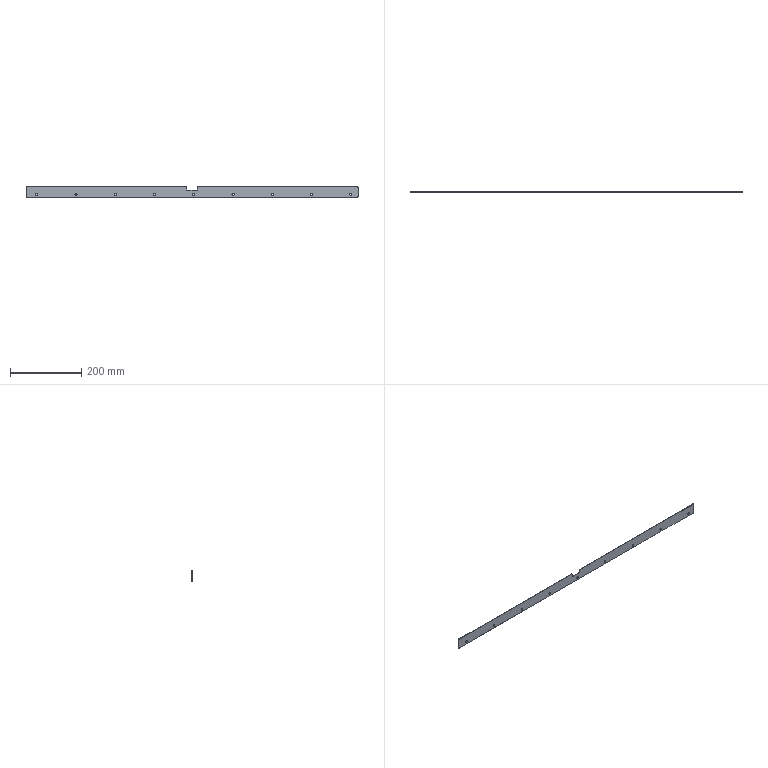Part | NX | features solid 2 | 1 solid | 34 faces | box 930 x 1.5 x 30 mm | volume 41011 mm3 | cylinder 24 | plane 10 | commonest cylinder face diameters 6 x18 4 x6
STEP:
#1=CARTESIAN_POINT('',(629.,-1449.,118.844));
#2=VERTEX_POINT('',#1);
#3=CARTESIAN_POINT('',(631.,-1449.,116.844));
#4=VERTEX_POINT('',#3);
#5=CARTESIAN_POINT('',(629.,-1449.,116.844));
#6=DIRECTION('',(0.,1.,0.));
#7=DIRECTION('',(-1.,0.,0.));
#8=AXIS2_PLACEMENT_3D('',#5,#6,#7);
#9=CIRCLE('',#8,2.);
#10=EDGE_CURVE('',#2,#4,#9,.T.);
#11=ORIENTED_EDGE('',*,*,#10,.F.);
#12=CARTESIAN_POINT('',(629.,-1450.5,118.844));
#13=VERTEX_POINT('',#12);
#14=CARTESIAN_POINT('',(629.,-1449.,118.844));
#15=DIRECTION('',(0.,1.,0.));
#16=VECTOR('',#15,1000.);
#17=LINE('',#14,#16);
#18=EDGE_CURVE('',#13,#2,#17,.T.);
#19=ORIENTED_EDGE('',*,*,#18,.F.);
#20=CARTESIAN_POINT('',(631.,-1450.5,116.844));
#21=VERTEX_POINT('',#20);
#22=CARTESIAN_POINT('',(629.,-1450.5,116.844));
#23=DIRECTION('',(0.,-1.,0.));
#24=DIRECTION('',(-1.,0.,0.));
#25=AXIS2_PLACEMENT_3D('',#22,#23,#24);
#26=CIRCLE('',#25,2.);
#27=EDGE_CURVE('',#21,#13,#26,.T.);
#28=ORIENTED_EDGE('',*,*,#27,.F.);
#29=CARTESIAN_POINT('',(631.,-1449.,116.844));
#30=DIRECTION('',(0.,-1.,0.));
#31=VECTOR('',#30,1000.);
#32=LINE('',#29,#31);
#33=EDGE_CURVE('',#4,#21,#32,.T.);
#34=ORIENTED_EDGE('',*,*,#33,.F.);
#35=EDGE_LOOP('',(#11,#19,#28,#34));
#36=FACE_BOUND('',#35,.T.);
#37=CARTESIAN_POINT('',(629.,-1449.,116.844));
#38=DIRECTION('',(0.,-1.,0.));
#39=DIRECTION('',(0.,0.,-1.));
#40=AXIS2_PLACEMENT_3D('',#37,#38,#39);
#41=CYLINDRICAL_SURFACE('',#40,2.);
#42=ADVANCED_FACE('',(#36),#41,.T.);
#43=CARTESIAN_POINT('',(631.,-1449.,90.844));
#44=VERTEX_POINT('',#43);
#45=CARTESIAN_POINT('',(629.,-1449.,88.844));
#46=VERTEX_POINT('',#45);
#47=CARTESIAN_POINT('',(629.,-1449.,90.844));
#48=DIRECTION('',(0.,1.,0.));
#49=DIRECTION('',(-1.,0.,0.));
#50=AXIS2_PLACEMENT_3D('',#47,#48,#49);
#51=CIRCLE('',#50,2.);
#52=EDGE_CURVE('',#44,#46,#51,.T.);
#53=ORIENTED_EDGE('',*,*,#52,.F.);
#54=CARTESIAN_POINT('',(631.,-1450.5,90.844));
#55=VERTEX_POINT('',#54);
#56=CARTESIAN_POINT('',(631.,-1449.,90.844));
#57=DIRECTION('',(0.,1.,0.));
#58=VECTOR('',#57,1000.);
#59=LINE('',#56,#58);
#60=EDGE_CURVE('',#55,#44,#59,.T.);
#61=ORIENTED_EDGE('',*,*,#60,.F.);
#62=CARTESIAN_POINT('',(629.,-1450.5,88.844));
#63=VERTEX_POINT('',#62);
#64=CARTESIAN_POINT('',(629.,-1450.5,90.844));
#65=DIRECTION('',(0.,-1.,0.));
#66=DIRECTION('',(-1.,0.,0.));
#67=AXIS2_PLACEMENT_3D('',#64,#65,#66);
#68=CIRCLE('',#67,2.);
#69=EDGE_CURVE('',#63,#55,#68,.T.);
#70=ORIENTED_EDGE('',*,*,#69,.F.);
#71=CARTESIAN_POINT('',(629.,-1449.,88.844));
#72=DIRECTION('',(0.,-1.,0.));
#73=VECTOR('',#72,1000.);
#74=LINE('',#71,#73);
#75=EDGE_CURVE('',#46,#63,#74,.T.);
#76=ORIENTED_EDGE('',*,*,#75,.F.);
#77=EDGE_LOOP('',(#53,#61,#70,#76));
#78=FACE_BOUND('',#77,.T.);
#79=CARTESIAN_POINT('',(629.,-1449.,90.844));
#80=DIRECTION('',(0.,-1.,0.));
#81=DIRECTION('',(0.,0.,-1.));
#82=AXIS2_PLACEMENT_3D('',#79,#80,#81);
#83=CYLINDRICAL_SURFACE('',#82,2.);
#84=ADVANCED_FACE('',(#78),#83,.T.);
#85=CARTESIAN_POINT('',(149.,-1449.,118.844));
#86=VERTEX_POINT('',#85);
#87=CARTESIAN_POINT('',(151.,-1449.,116.844));
#88=VERTEX_POINT('',#87);
#89=CARTESIAN_POINT('',(149.,-1449.,116.844));
#90=DIRECTION('',(0.,1.,0.));
#91=DIRECTION('',(-1.,0.,0.));
#92=AXIS2_PLACEMENT_3D('',#89,#90,#91);
#93=CIRCLE('',#92,2.);
#94=EDGE_CURVE('',#86,#88,#93,.T.);
#95=ORIENTED_EDGE('',*,*,#94,.F.);
#96=CARTESIAN_POINT('',(149.,-1450.5,118.844));
#97=VERTEX_POINT('',#96);
#98=CARTESIAN_POINT('',(149.,-1449.,118.844));
#99=DIRECTION('',(0.,1.,0.));
#100=VECTOR('',#99,1000.);
#101=LINE('',#98,#100);
#102=EDGE_CURVE('',#97,#86,#101,.T.);
#103=ORIENTED_EDGE('',*,*,#102,.F.);
#104=CARTESIAN_POINT('',(151.,-1450.5,116.844));
#105=VERTEX_POINT('',#104);
#106=CARTESIAN_POINT('',(149.,-1450.5,116.844));
#107=DIRECTION('',(0.,-1.,0.));
#108=DIRECTION('',(-1.,0.,0.));
#109=AXIS2_PLACEMENT_3D('',#106,#107,#108);
#110=CIRCLE('',#109,2.);
#111=EDGE_CURVE('',#105,#97,#110,.T.);
#112=ORIENTED_EDGE('',*,*,#111,.F.);
#113=CARTESIAN_POINT('',(151.,-1450.5,116.844));
#114=DIRECTION('',(0.,-1.,0.));
#115=VECTOR('',#114,1000.);
#116=LINE('',#113,#115);
#117=EDGE_CURVE('',#88,#105,#116,.T.);
#118=ORIENTED_EDGE('',*,*,#117,.F.);
#119=EDGE_LOOP('',(#95,#103,#112,#118));
#120=FACE_BOUND('',#119,.T.);
#121=CARTESIAN_POINT('',(149.,-1450.5,116.844));
#122=DIRECTION('',(0.,-1.,0.));
#123=DIRECTION('',(1.,0.,0.));
#124=AXIS2_PLACEMENT_3D('',#121,#122,#123);
#125=CYLINDRICAL_SURFACE('',#124,2.);
#126=ADVANCED_FACE('',(#120),#125,.T.);
#127=CARTESIAN_POINT('',(181.,-1449.,116.844));
#128=VERTEX_POINT('',#127);
#129=CARTESIAN_POINT('',(183.,-1449.,118.844));
#130=VERTEX_POINT('',#129);
#131=CARTESIAN_POINT('',(183.,-1449.,116.844));
#132=DIRECTION('',(0.,1.,0.));
#133=DIRECTION('',(-1.,0.,0.));
#134=AXIS2_PLACEMENT_3D('',#131,#132,#133);
#135=CIRCLE('',#134,2.);
#136=EDGE_CURVE('',#128,#130,#135,.T.);
#137=ORIENTED_EDGE('',*,*,#136,.F.);
#138=CARTESIAN_POINT('',(181.,-1450.5,116.844));
#139=VERTEX_POINT('',#138);
#140=CARTESIAN_POINT('',(181.,-1450.5,116.844));
#141=DIRECTION('',(0.,1.,0.));
#142=VECTOR('',#141,1000.);
#143=LINE('',#140,#142);
#144=EDGE_CURVE('',#139,#128,#143,.T.);
#145=ORIENTED_EDGE('',*,*,#144,.F.);
#146=CARTESIAN_POINT('',(183.,-1450.5,118.844));
#147=VERTEX_POINT('',#146);
#148=CARTESIAN_POINT('',(183.,-1450.5,116.844));
#149=DIRECTION('',(0.,-1.,0.));
#150=DIRECTION('',(-1.,0.,0.));
#151=AXIS2_PLACEMENT_3D('',#148,#149,#150);
#152=CIRCLE('',#151,2.);
#153=EDGE_CURVE('',#147,#139,#152,.T.);
#154=ORIENTED_EDGE('',*,*,#153,.F.);
#155=CARTESIAN_POINT('',(183.,-1449.,118.844));
#156=DIRECTION('',(0.,-1.,0.));
#157=VECTOR('',#156,1000.);
#158=LINE('',#155,#157);
#159=EDGE_CURVE('',#130,#147,#158,.T.);
#160=ORIENTED_EDGE('',*,*,#159,.F.);
#161=EDGE_LOOP('',(#137,#145,#154,#160));
#162=FACE_BOUND('',#161,.T.);
#163=CARTESIAN_POINT('',(183.,-1449.,116.844));
#164=DIRECTION('',(0.,-1.,0.));
#165=DIRECTION('',(1.,0.,0.));
#166=AXIS2_PLACEMENT_3D('',#163,#164,#165);
#167=CYLINDRICAL_SURFACE('',#166,2.);
#168=ADVANCED_FACE('',(#162),#167,.T.);
#169=CARTESIAN_POINT('',(-299.,-1449.,116.844));
#170=VERTEX_POINT('',#169);
#171=CARTESIAN_POINT('',(-297.,-1449.,118.844));
#172=VERTEX_POINT('',#171);
#173=CARTESIAN_POINT('',(-297.,-1449.,116.844));
#174=DIRECTION('',(0.,1.,0.));
#175=DIRECTION('',(-1.,0.,0.));
#176=AXIS2_PLACEMENT_3D('',#173,#174,#175);
#177=CIRCLE('',#176,2.);
#178=EDGE_CURVE('',#170,#172,#177,.T.);
#179=ORIENTED_EDGE('',*,*,#178,.F.);
#180=CARTESIAN_POINT('',(-299.,-1450.5,116.844));
#181=VERTEX_POINT('',#180);
#182=CARTESIAN_POINT('',(-299.,-1449.,116.844));
#183=DIRECTION('',(0.,1.,0.));
#184=VECTOR('',#183,1000.);
#185=LINE('',#182,#184);
#186=EDGE_CURVE('',#181,#170,#185,.T.);
#187=ORIENTED_EDGE('',*,*,#186,.F.);
#188=CARTESIAN_POINT('',(-297.,-1450.5,118.844));
#189=VERTEX_POINT('',#188);
#190=CARTESIAN_POINT('',(-297.,-1450.5,116.844));
#191=DIRECTION('',(0.,-1.,0.));
#192=DIRECTION('',(-1.,0.,0.));
#193=AXIS2_PLACEMENT_3D('',#190,#191,#192);
#194=CIRCLE('',#193,2.);
#195=EDGE_CURVE('',#189,#181,#194,.T.);
#196=ORIENTED_EDGE('',*,*,#195,.F.);
#197=CARTESIAN_POINT('',(-297.,-1449.,118.844));
#198=DIRECTION('',(0.,-1.,0.));
#199=VECTOR('',#198,1000.);
#200=LINE('',#197,#199);
#201=EDGE_CURVE('',#172,#189,#200,.T.);
#202=ORIENTED_EDGE('',*,*,#201,.F.);
#203=EDGE_LOOP('',(#179,#187,#196,#202));
#204=FACE_BOUND('',#203,.T.);
#205=CARTESIAN_POINT('',(-297.,-1449.,116.844));
#206=DIRECTION('',(0.,-1.,0.));
#207=DIRECTION('',(0.,0.,-1.));
#208=AXIS2_PLACEMENT_3D('',#205,#206,#207);
#209=CYLINDRICAL_SURFACE('',#208,2.);
#210=ADVANCED_FACE('',(#204),#209,.T.);
#211=CARTESIAN_POINT('',(-297.,-1449.,88.844));
#212=VERTEX_POINT('',#211);
#213=CARTESIAN_POINT('',(-299.,-1449.,90.844));
#214=VERTEX_POINT('',#213);
#215=CARTESIAN_POINT('',(-297.,-1449.,90.844));
#216=DIRECTION('',(0.,1.,0.));
#217=DIRECTION('',(-1.,0.,0.));
#218=AXIS2_PLACEMENT_3D('',#215,#216,#217);
#219=CIRCLE('',#218,2.);
#220=EDGE_CURVE('',#212,#214,#219,.T.);
#221=ORIENTED_EDGE('',*,*,#220,.F.);
#222=CARTESIAN_POINT('',(-297.,-1450.5,88.844));
#223=VERTEX_POINT('',#222);
#224=CARTESIAN_POINT('',(-297.,-1449.,88.844));
#225=DIRECTION('',(0.,1.,0.));
#226=VECTOR('',#225,1000.);
#227=LINE('',#224,#226);
#228=EDGE_CURVE('',#223,#212,#227,.T.);
#229=ORIENTED_EDGE('',*,*,#228,.F.);
#230=CARTESIAN_POINT('',(-299.,-1450.5,90.844));
#231=VERTEX_POINT('',#230);
#232=CARTESIAN_POINT('',(-297.,-1450.5,90.844));
#233=DIRECTION('',(0.,-1.,0.));
#234=DIRECTION('',(-1.,0.,0.));
#235=AXIS2_PLACEMENT_3D('',#232,#233,#234);
#236=CIRCLE('',#235,2.);
#237=EDGE_CURVE('',#231,#223,#236,.T.);
#238=ORIENTED_EDGE('',*,*,#237,.F.);
#239=CARTESIAN_POINT('',(-299.,-1449.,90.844));
#240=DIRECTION('',(0.,-1.,0.));
#241=VECTOR('',#240,1000.);
#242=LINE('',#239,#241);
#243=EDGE_CURVE('',#214,#231,#242,.T.);
#244=ORIENTED_EDGE('',*,*,#243,.F.);
#245=EDGE_LOOP('',(#221,#229,#238,#244));
#246=FACE_BOUND('',#245,.T.);
#247=CARTESIAN_POINT('',(-297.,-1449.,90.844));
#248=DIRECTION('',(0.,-1.,0.));
#249=DIRECTION('',(0.,0.,-1.));
#250=AXIS2_PLACEMENT_3D('',#247,#248,#249);
#251=CYLINDRICAL_SURFACE('',#250,2.);
#252=ADVANCED_FACE('',(#246),#251,.T.);
#253=CARTESIAN_POINT('',(-266.,-1450.5,97.344));
#254=VERTEX_POINT('',#253);
#255=CARTESIAN_POINT('',(-266.,-1449.,97.344));
#256=VERTEX_POINT('',#255);
#257=CARTESIAN_POINT('',(-266.,-2379.485,97.344));
#258=DIRECTION('',(0.,1.,0.));
#259=VECTOR('',#258,1000.);
#260=LINE('',#257,#259);
#261=EDGE_CURVE('',#254,#256,#260,.T.);
#262=ORIENTED_EDGE('',*,*,#261,.F.);
#263=CARTESIAN_POINT('',(-272.,-1450.5,97.344));
#264=VERTEX_POINT('',#263);
#265=CARTESIAN_POINT('',(-269.,-1450.5,97.344));
#266=DIRECTION('',(0.,1.,0.));
#267=DIRECTION('',(-1.,0.,0.));
#268=AXIS2_PLACEMENT_3D('',#265,#266,#267);
#269=CIRCLE('',#268,3.);
#270=EDGE_CURVE('',#264,#254,#269,.T.);
#271=ORIENTED_EDGE('',*,*,#270,.F.);
#272=CARTESIAN_POINT('',(-272.,-1449.,97.344));
#273=VERTEX_POINT('',#272);
#274=CARTESIAN_POINT('',(-272.,-2379.485,97.344));
#275=DIRECTION('',(0.,1.,0.));
#276=VECTOR('',#275,1000.);
#277=LINE('',#274,#276);
#278=EDGE_CURVE('',#273,#264,#277,.F.);
#279=ORIENTED_EDGE('',*,*,#278,.F.);
#280=CARTESIAN_POINT('',(-269.,-1449.,97.344));
#281=DIRECTION('',(0.,1.,0.));
#282=DIRECTION('',(-1.,0.,0.));
#283=AXIS2_PLACEMENT_3D('',#280,#281,#282);
#284=CIRCLE('',#283,3.);
#285=EDGE_CURVE('',#273,#256,#284,.T.);
#286=ORIENTED_EDGE('',*,*,#285,.T.);
#287=EDGE_LOOP('',(#262,#271,#279,#286));
#288=FACE_BOUND('',#287,.T.);
#289=CARTESIAN_POINT('',(-269.,-2379.485,97.344));
#290=DIRECTION('',(0.,1.,0.));
#291=DIRECTION('',(-1.,0.,0.));
#292=AXIS2_PLACEMENT_3D('',#289,#290,#291);
#293=CYLINDRICAL_SURFACE('',#292,3.);
#294=ADVANCED_FACE('',(#288),#293,.F.);
#295=CARTESIAN_POINT('',(-156.,-1450.5,97.344));
#296=VERTEX_POINT('',#295);
#297=CARTESIAN_POINT('',(-156.,-1449.,97.344));
#298=VERTEX_POINT('',#297);
#299=CARTESIAN_POINT('',(-156.,-2379.485,97.344));
#300=DIRECTION('',(0.,1.,0.));
#301=VECTOR('',#300,1000.);
#302=LINE('',#299,#301);
#303=EDGE_CURVE('',#296,#298,#302,.T.);
#304=ORIENTED_EDGE('',*,*,#303,.F.);
#305=CARTESIAN_POINT('',(-162.,-1450.5,97.344));
#306=VERTEX_POINT('',#305);
#307=CARTESIAN_POINT('',(-159.,-1450.5,97.344));
#308=DIRECTION('',(0.,1.,0.));
#309=DIRECTION('',(-1.,0.,0.));
#310=AXIS2_PLACEMENT_3D('',#307,#308,#309);
#311=CIRCLE('',#310,3.);
#312=EDGE_CURVE('',#306,#296,#311,.T.);
#313=ORIENTED_EDGE('',*,*,#312,.F.);
#314=CARTESIAN_POINT('',(-162.,-1449.,97.344));
#315=VERTEX_POINT('',#314);
#316=CARTESIAN_POINT('',(-162.,-2379.485,97.344));
#317=DIRECTION('',(0.,1.,0.));
#318=VECTOR('',#317,1000.);
#319=LINE('',#316,#318);
#320=EDGE_CURVE('',#315,#306,#319,.F.);
#321=ORIENTED_EDGE('',*,*,#320,.F.);
#322=CARTESIAN_POINT('',(-159.,-1449.,97.344));
#323=DIRECTION('',(0.,1.,0.));
#324=DIRECTION('',(-1.,0.,0.));
#325=AXIS2_PLACEMENT_3D('',#322,#323,#324);
#326=CIRCLE('',#325,3.);
#327=EDGE_CURVE('',#315,#298,#326,.T.);
#328=ORIENTED_EDGE('',*,*,#327,.T.);
#329=EDGE_LOOP('',(#304,#313,#321,#328));
#330=FACE_BOUND('',#329,.T.);
#331=CARTESIAN_POINT('',(-159.,-2379.485,97.344));
#332=DIRECTION('',(0.,1.,0.));
#333=DIRECTION('',(-1.,0.,0.));
#334=AXIS2_PLACEMENT_3D('',#331,#332,#333);
#335=CYLINDRICAL_SURFACE('',#334,3.);
#336=ADVANCED_FACE('',(#330),#335,.F.);
#337=CARTESIAN_POINT('',(-46.,-1449.,97.344));
#338=VERTEX_POINT('',#337);
#339=CARTESIAN_POINT('',(-46.,-1450.5,97.344));
#340=VERTEX_POINT('',#339);
#341=CARTESIAN_POINT('',(-46.,-2379.485,97.344));
#342=DIRECTION('',(0.,1.,0.));
#343=VECTOR('',#342,1000.);
#344=LINE('',#341,#343);
#345=EDGE_CURVE('',#338,#340,#344,.F.);
#346=ORIENTED_EDGE('',*,*,#345,.T.);
#347=CARTESIAN_POINT('',(-52.,-1450.5,97.344));
#348=VERTEX_POINT('',#347);
#349=CARTESIAN_POINT('',(-49.,-1450.5,97.344));
#350=DIRECTION('',(0.,1.,0.));
#351=DIRECTION('',(-1.,0.,0.));
#352=AXIS2_PLACEMENT_3D('',#349,#350,#351);
#353=CIRCLE('',#352,3.);
#354=EDGE_CURVE('',#348,#340,#353,.T.);
#355=ORIENTED_EDGE('',*,*,#354,.F.);
#356=CARTESIAN_POINT('',(-52.,-1449.,97.344));
#357=VERTEX_POINT('',#356);
#358=CARTESIAN_POINT('',(-52.,-2379.485,97.344));
#359=DIRECTION('',(0.,1.,0.));
#360=VECTOR('',#359,1000.);
#361=LINE('',#358,#360);
#362=EDGE_CURVE('',#348,#357,#361,.T.);
#363=ORIENTED_EDGE('',*,*,#362,.T.);
#364=CARTESIAN_POINT('',(-49.,-1449.,97.344));
#365=DIRECTION('',(0.,1.,0.));
#366=DIRECTION('',(-1.,0.,0.));
#367=AXIS2_PLACEMENT_3D('',#364,#365,#366);
#368=CIRCLE('',#367,3.);
#369=EDGE_CURVE('',#357,#338,#368,.T.);
#370=ORIENTED_EDGE('',*,*,#369,.T.);
#371=EDGE_LOOP('',(#346,#355,#363,#370));
#372=FACE_BOUND('',#371,.T.);
#373=CARTESIAN_POINT('',(-49.,-2379.485,97.344));
#374=DIRECTION('',(0.,1.,0.));
#375=DIRECTION('',(-1.,0.,0.));
#376=AXIS2_PLACEMENT_3D('',#373,#374,#375);
#377=CYLINDRICAL_SURFACE('',#376,3.);
#378=ADVANCED_FACE('',(#372),#377,.F.);
#379=CARTESIAN_POINT('',(64.,-1450.5,97.344));
#380=VERTEX_POINT('',#379);
#381=CARTESIAN_POINT('',(64.,-1449.,97.344));
#382=VERTEX_POINT('',#381);
#383=CARTESIAN_POINT('',(64.,-2379.485,97.344));
#384=DIRECTION('',(0.,1.,0.));
#385=VECTOR('',#384,1000.);
#386=LINE('',#383,#385);
#387=EDGE_CURVE('',#380,#382,#386,.T.);
#388=ORIENTED_EDGE('',*,*,#387,.F.);
#389=CARTESIAN_POINT('',(58.,-1450.5,97.344));
#390=VERTEX_POINT('',#389);
#391=CARTESIAN_POINT('',(61.,-1450.5,97.344));
#392=DIRECTION('',(0.,1.,0.));
#393=DIRECTION('',(-1.,0.,0.));
#394=AXIS2_PLACEMENT_3D('',#391,#392,#393);
#395=CIRCLE('',#394,3.);
#396=EDGE_CURVE('',#390,#380,#395,.T.);
#397=ORIENTED_EDGE('',*,*,#396,.F.);
#398=CARTESIAN_POINT('',(58.,-1449.,97.344));
#399=VERTEX_POINT('',#398);
#400=CARTESIAN_POINT('',(58.,-2379.485,97.344));
#401=DIRECTION('',(0.,1.,0.));
#402=VECTOR('',#401,1000.);
#403=LINE('',#400,#402);
#404=EDGE_CURVE('',#399,#390,#403,.F.);
#405=ORIENTED_EDGE('',*,*,#404,.F.);
#406=CARTESIAN_POINT('',(61.,-1449.,97.344));
#407=DIRECTION('',(0.,1.,0.));
#408=DIRECTION('',(-1.,0.,0.));
#409=AXIS2_PLACEMENT_3D('',#406,#407,#408);
#410=CIRCLE('',#409,3.);
#411=EDGE_CURVE('',#399,#382,#410,.T.);
#412=ORIENTED_EDGE('',*,*,#411,.T.);
#413=EDGE_LOOP('',(#388,#397,#405,#412));
#414=FACE_BOUND('',#413,.T.);
#415=CARTESIAN_POINT('',(61.,-2379.485,97.344));
#416=DIRECTION('',(0.,1.,0.));
#417=DIRECTION('',(-1.,0.,0.));
#418=AXIS2_PLACEMENT_3D('',#415,#416,#417);
#419=CYLINDRICAL_SURFACE('',#418,3.);
#420=ADVANCED_FACE('',(#414),#419,.F.);
#421=CARTESIAN_POINT('',(174.,-1450.5,97.344));
#422=VERTEX_POINT('',#421);
#423=CARTESIAN_POINT('',(174.,-1449.,97.344));
#424=VERTEX_POINT('',#423);
#425=CARTESIAN_POINT('',(174.,-2379.485,97.344));
#426=DIRECTION('',(0.,1.,0.));
#427=VECTOR('',#426,1000.);
#428=LINE('',#425,#427);
#429=EDGE_CURVE('',#422,#424,#428,.T.);
#430=ORIENTED_EDGE('',*,*,#429,.F.);
#431=CARTESIAN_POINT('',(168.,-1450.5,97.344));
#432=VERTEX_POINT('',#431);
#433=CARTESIAN_POINT('',(171.,-1450.5,97.344));
#434=DIRECTION('',(0.,1.,0.));
#435=DIRECTION('',(-1.,0.,0.));
#436=AXIS2_PLACEMENT_3D('',#433,#434,#435);
#437=CIRCLE('',#436,3.);
#438=EDGE_CURVE('',#432,#422,#437,.T.);
#439=ORIENTED_EDGE('',*,*,#438,.F.);
#440=CARTESIAN_POINT('',(168.,-1449.,97.344));
#441=VERTEX_POINT('',#440);
#442=CARTESIAN_POINT('',(168.,-2379.485,97.344));
#443=DIRECTION('',(0.,1.,0.));
#444=VECTOR('',#443,1000.);
#445=LINE('',#442,#444);
#446=EDGE_CURVE('',#441,#432,#445,.F.);
#447=ORIENTED_EDGE('',*,*,#446,.F.);
#448=CARTESIAN_POINT('',(171.,-1449.,97.344));
#449=DIRECTION('',(0.,1.,0.));
#450=DIRECTION('',(-1.,0.,0.));
#451=AXIS2_PLACEMENT_3D('',#448,#449,#450);
#452=CIRCLE('',#451,3.);
#453=EDGE_CURVE('',#441,#424,#452,.T.);
#454=ORIENTED_EDGE('',*,*,#453,.T.);
#455=EDGE_LOOP('',(#430,#439,#447,#454));
#456=FACE_BOUND('',#455,.T.);
#457=CARTESIAN_POINT('',(171.,-2379.485,97.344));
#458=DIRECTION('',(0.,1.,0.));
#459=DIRECTION('',(-1.,0.,0.));
#460=AXIS2_PLACEMENT_3D('',#457,#458,#459);
#461=CYLINDRICAL_SURFACE('',#460,3.);
#462=ADVANCED_FACE('',(#456),#461,.F.);
#463=CARTESIAN_POINT('',(284.,-1449.,97.344));
#464=VERTEX_POINT('',#463);
#465=CARTESIAN_POINT('',(284.,-1450.5,97.344));
#466=VERTEX_POINT('',#465);
#467=CARTESIAN_POINT('',(284.,-2379.485,97.344));
#468=DIRECTION('',(0.,1.,0.));
#469=VECTOR('',#468,1000.);
#470=LINE('',#467,#469);
#471=EDGE_CURVE('',#464,#466,#470,.F.);
#472=ORIENTED_EDGE('',*,*,#471,.T.);
#473=CARTESIAN_POINT('',(278.,-1450.5,97.344));
#474=VERTEX_POINT('',#473);
#475=CARTESIAN_POINT('',(281.,-1450.5,97.344));
#476=DIRECTION('',(0.,1.,0.));
#477=DIRECTION('',(-1.,0.,0.));
#478=AXIS2_PLACEMENT_3D('',#475,#476,#477);
#479=CIRCLE('',#478,3.);
#480=EDGE_CURVE('',#474,#466,#479,.T.);
#481=ORIENTED_EDGE('',*,*,#480,.F.);
#482=CARTESIAN_POINT('',(278.,-1449.,97.344));
#483=VERTEX_POINT('',#482);
#484=CARTESIAN_POINT('',(278.,-2379.485,97.344));
#485=DIRECTION('',(0.,1.,0.));
#486=VECTOR('',#485,1000.);
#487=LINE('',#484,#486);
#488=EDGE_CURVE('',#474,#483,#487,.T.);
#489=ORIENTED_EDGE('',*,*,#488,.T.);
#490=CARTESIAN_POINT('',(281.,-1449.,97.344));
#491=DIRECTION('',(0.,1.,0.));
#492=DIRECTION('',(-1.,0.,0.));
#493=AXIS2_PLACEMENT_3D('',#490,#491,#492);
#494=CIRCLE('',#493,3.);
#495=EDGE_CURVE('',#483,#464,#494,.T.);
#496=ORIENTED_EDGE('',*,*,#495,.T.);
#497=EDGE_LOOP('',(#472,#481,#489,#496));
#498=FACE_BOUND('',#497,.T.);
#499=CARTESIAN_POINT('',(281.,-2379.485,97.344));
#500=DIRECTION('',(0.,1.,0.));
#501=DIRECTION('',(-1.,0.,0.));
#502=AXIS2_PLACEMENT_3D('',#499,#500,#501);
#503=CYLINDRICAL_SURFACE('',#502,3.);
#504=ADVANCED_FACE('',(#498),#503,.F.);
#505=CARTESIAN_POINT('',(394.,-1450.5,97.344));
#506=VERTEX_POINT('',#505);
#507=CARTESIAN_POINT('',(394.,-1449.,97.344));
#508=VERTEX_POINT('',#507);
#509=CARTESIAN_POINT('',(394.,-2379.485,97.344));
#510=DIRECTION('',(0.,1.,0.));
#511=VECTOR('',#510,1000.);
#512=LINE('',#509,#511);
#513=EDGE_CURVE('',#506,#508,#512,.T.);
#514=ORIENTED_EDGE('',*,*,#513,.F.);
#515=CARTESIAN_POINT('',(388.,-1450.5,97.344));
#516=VERTEX_POINT('',#515);
#517=CARTESIAN_POINT('',(391.,-1450.5,97.344));
#518=DIRECTION('',(0.,1.,0.));
#519=DIRECTION('',(-1.,0.,0.));
#520=AXIS2_PLACEMENT_3D('',#517,#518,#519);
#521=CIRCLE('',#520,3.);
#522=EDGE_CURVE('',#516,#506,#521,.T.);
#523=ORIENTED_EDGE('',*,*,#522,.F.);
#524=CARTESIAN_POINT('',(388.,-1449.,97.344));
#525=VERTEX_POINT('',#524);
#526=CARTESIAN_POINT('',(388.,-2379.485,97.344));
#527=DIRECTION('',(0.,1.,0.));
#528=VECTOR('',#527,1000.);
#529=LINE('',#526,#528);
#530=EDGE_CURVE('',#525,#516,#529,.F.);
#531=ORIENTED_EDGE('',*,*,#530,.F.);
#532=CARTESIAN_POINT('',(391.,-1449.,97.344));
#533=DIRECTION('',(0.,1.,0.));
#534=DIRECTION('',(-1.,0.,0.));
#535=AXIS2_PLACEMENT_3D('',#532,#533,#534);
#536=CIRCLE('',#535,3.);
#537=EDGE_CURVE('',#525,#508,#536,.T.);
#538=ORIENTED_EDGE('',*,*,#537,.T.);
#539=EDGE_LOOP('',(#514,#523,#531,#538));
#540=FACE_BOUND('',#539,.T.);
#541=CARTESIAN_POINT('',(391.,-2379.485,97.344));
#542=DIRECTION('',(0.,1.,0.));
#543=DIRECTION('',(-1.,0.,0.));
#544=AXIS2_PLACEMENT_3D('',#541,#542,#543);
#545=CYLINDRICAL_SURFACE('',#544,3.);
#546=ADVANCED_FACE('',(#540),#545,.F.);
#547=CARTESIAN_POINT('',(504.,-1449.,97.344));
#548=VERTEX_POINT('',#547);
#549=CARTESIAN_POINT('',(504.,-1450.5,97.344));
#550=VERTEX_POINT('',#549);
#551=CARTESIAN_POINT('',(504.,-2379.485,97.344));
#552=DIRECTION('',(0.,1.,0.));
#553=VECTOR('',#552,1000.);
#554=LINE('',#551,#553);
#555=EDGE_CURVE('',#548,#550,#554,.F.);
#556=ORIENTED_EDGE('',*,*,#555,.T.);
#557=CARTESIAN_POINT('',(498.,-1450.5,97.344));
#558=VERTEX_POINT('',#557);
#559=CARTESIAN_POINT('',(501.,-1450.5,97.344));
#560=DIRECTION('',(0.,1.,0.));
#561=DIRECTION('',(-1.,0.,0.));
#562=AXIS2_PLACEMENT_3D('',#559,#560,#561);
#563=CIRCLE('',#562,3.);
#564=EDGE_CURVE('',#558,#550,#563,.T.);
#565=ORIENTED_EDGE('',*,*,#564,.F.);
#566=CARTESIAN_POINT('',(498.,-1449.,97.344));
#567=VERTEX_POINT('',#566);
#568=CARTESIAN_POINT('',(498.,-2379.485,97.344));
#569=DIRECTION('',(0.,1.,0.));
#570=VECTOR('',#569,1000.);
#571=LINE('',#568,#570);
#572=EDGE_CURVE('',#558,#567,#571,.T.);
#573=ORIENTED_EDGE('',*,*,#572,.T.);
#574=CARTESIAN_POINT('',(501.,-1449.,97.344));
#575=DIRECTION('',(0.,1.,0.));
#576=DIRECTION('',(-1.,0.,0.));
#577=AXIS2_PLACEMENT_3D('',#574,#575,#576);
#578=CIRCLE('',#577,3.);
#579=EDGE_CURVE('',#567,#548,#578,.T.);
#580=ORIENTED_EDGE('',*,*,#579,.T.);
#581=EDGE_LOOP('',(#556,#565,#573,#580));
#582=FACE_BOUND('',#581,.T.);
#583=CARTESIAN_POINT('',(501.,-2379.485,97.344));
#584=DIRECTION('',(0.,1.,0.));
#585=DIRECTION('',(-1.,0.,0.));
#586=AXIS2_PLACEMENT_3D('',#583,#584,#585);
#587=CYLINDRICAL_SURFACE('',#586,3.);
#588=ADVANCED_FACE('',(#582),#587,.F.);
#589=CARTESIAN_POINT('',(614.,-1450.5,97.344));
#590=VERTEX_POINT('',#589);
#591=CARTESIAN_POINT('',(614.,-1449.,97.344));
#592=VERTEX_POINT('',#591);
#593=CARTESIAN_POINT('',(614.,-2379.485,97.344));
#594=DIRECTION('',(0.,1.,0.));
#595=VECTOR('',#594,1000.);
#596=LINE('',#593,#595);
#597=EDGE_CURVE('',#590,#592,#596,.T.);
#598=ORIENTED_EDGE('',*,*,#597,.F.);
#599=CARTESIAN_POINT('',(608.,-1450.5,97.344));
#600=VERTEX_POINT('',#599);
#601=CARTESIAN_POINT('',(611.,-1450.5,97.344));
#602=DIRECTION('',(0.,1.,0.));
#603=DIRECTION('',(-1.,0.,0.));
#604=AXIS2_PLACEMENT_3D('',#601,#602,#603);
#605=CIRCLE('',#604,3.);
#606=EDGE_CURVE('',#600,#590,#605,.T.);
#607=ORIENTED_EDGE('',*,*,#606,.F.);
#608=CARTESIAN_POINT('',(608.,-1449.,97.344));
#609=VERTEX_POINT('',#608);
#610=CARTESIAN_POINT('',(608.,-2379.485,97.344));
#611=DIRECTION('',(0.,1.,0.));
#612=VECTOR('',#611,1000.);
#613=LINE('',#610,#612);
#614=EDGE_CURVE('',#609,#600,#613,.F.);
#615=ORIENTED_EDGE('',*,*,#614,.F.);
#616=CARTESIAN_POINT('',(611.,-1449.,97.344));
#617=DIRECTION('',(0.,1.,0.));
#618=DIRECTION('',(-1.,0.,0.));
#619=AXIS2_PLACEMENT_3D('',#616,#617,#618);
#620=CIRCLE('',#619,3.);
#621=EDGE_CURVE('',#609,#592,#620,.T.);
#622=ORIENTED_EDGE('',*,*,#621,.T.);
#623=EDGE_LOOP('',(#598,#607,#615,#622));
#624=FACE_BOUND('',#623,.T.);
#625=CARTESIAN_POINT('',(611.,-2379.485,97.344));
#626=DIRECTION('',(0.,1.,0.));
#627=DIRECTION('',(-1.,0.,0.));
#628=AXIS2_PLACEMENT_3D('',#625,#626,#627);
#629=CYLINDRICAL_SURFACE('',#628,3.);
#630=ADVANCED_FACE('',(#624),#629,.F.);
#631=CARTESIAN_POINT('',(181.,-1450.5,108.844));
#632=VERTEX_POINT('',#631);
#633=CARTESIAN_POINT('',(181.,-1450.5,118.844));
#634=DIRECTION('',(0.,0.,-1.));
#635=VECTOR('',#634,1000.);
#636=LINE('',#633,#635);
#637=EDGE_CURVE('',#139,#632,#636,.T.);
#638=ORIENTED_EDGE('',*,*,#637,.F.);
#639=ORIENTED_EDGE('',*,*,#144,.T.);
#640=CARTESIAN_POINT('',(181.,-1449.,108.844));
#641=VERTEX_POINT('',#640);
#642=CARTESIAN_POINT('',(181.,-1449.,118.844));
#643=DIRECTION('',(0.,0.,-1.));
#644=VECTOR('',#643,1000.);
#645=LINE('',#642,#644);
#646=EDGE_CURVE('',#128,#641,#645,.T.);
#647=ORIENTED_EDGE('',*,*,#646,.T.);
#648=CARTESIAN_POINT('',(181.,-1450.5,108.844));
#649=DIRECTION('',(0.,-1.,0.));
#650=VECTOR('',#649,1000.);
#651=LINE('',#648,#650);
#652=EDGE_CURVE('',#641,#632,#651,.T.);
#653=ORIENTED_EDGE('',*,*,#652,.T.);
#654=EDGE_LOOP('',(#638,#639,#647,#653));
#655=FACE_BOUND('',#654,.T.);
#656=CARTESIAN_POINT('',(181.,-1450.5,118.844));
#657=DIRECTION('',(1.,0.,0.));
#658=DIRECTION('',(0.,0.,1.));
#659=AXIS2_PLACEMENT_3D('',#656,#657,#658);
#660=PLANE('',#659);
#661=ADVANCED_FACE('',(#655),#660,.F.);
#662=CARTESIAN_POINT('',(151.,-1449.,108.844));
#663=VERTEX_POINT('',#662);
#664=CARTESIAN_POINT('',(151.,-1450.5,108.844));
#665=VERTEX_POINT('',#664);
#666=CARTESIAN_POINT('',(151.,-1450.5,108.844));
#667=DIRECTION('',(0.,-1.,0.));
#668=VECTOR('',#667,1000.);
#669=LINE('',#666,#668);
#670=EDGE_CURVE('',#663,#665,#669,.T.);
#671=ORIENTED_EDGE('',*,*,#670,.T.);
#672=CARTESIAN_POINT('',(-299.,-1450.5,108.844));
#673=DIRECTION('',(-1.,0.,0.));
#674=VECTOR('',#673,1000.);
#675=LINE('',#672,#674);
#676=EDGE_CURVE('',#632,#665,#675,.T.);
#677=ORIENTED_EDGE('',*,*,#676,.F.);
#678=ORIENTED_EDGE('',*,*,#652,.F.);
#679=CARTESIAN_POINT('',(-299.,-1449.,108.844));
#680=DIRECTION('',(-1.,0.,0.));
#681=VECTOR('',#680,1000.);
#682=LINE('',#679,#681);
#683=EDGE_CURVE('',#641,#663,#682,.T.);
#684=ORIENTED_EDGE('',*,*,#683,.T.);
#685=EDGE_LOOP('',(#671,#677,#678,#684));
#686=FACE_BOUND('',#685,.T.);
#687=CARTESIAN_POINT('',(-299.,-1450.5,108.844));
#688=DIRECTION('',(0.,0.,-1.));
#689=DIRECTION('',(0.,-1.,0.));
#690=AXIS2_PLACEMENT_3D('',#687,#688,#689);
#691=PLANE('',#690);
#692=ADVANCED_FACE('',(#686),#691,.F.);
#693=CARTESIAN_POINT('',(151.,-1449.,118.844));
#694=DIRECTION('',(0.,0.,1.));
#695=VECTOR('',#694,1000.);
#696=LINE('',#693,#695);
#697=EDGE_CURVE('',#663,#88,#696,.T.);
#698=ORIENTED_EDGE('',*,*,#697,.T.);
#699=ORIENTED_EDGE('',*,*,#117,.T.);
#700=CARTESIAN_POINT('',(151.,-1450.5,118.844));
#701=DIRECTION('',(0.,0.,1.));
#702=VECTOR('',#701,1000.);
#703=LINE('',#700,#702);
#704=EDGE_CURVE('',#665,#105,#703,.T.);
#705=ORIENTED_EDGE('',*,*,#704,.F.);
#706=ORIENTED_EDGE('',*,*,#670,.F.);
#707=EDGE_LOOP('',(#698,#699,#705,#706));
#708=FACE_BOUND('',#707,.T.);
#709=CARTESIAN_POINT('',(151.,-1450.5,118.844));
#710=DIRECTION('',(-1.,0.,0.));
#711=DIRECTION('',(0.,1.,0.));
#712=AXIS2_PLACEMENT_3D('',#709,#710,#711);
#713=PLANE('',#712);
#714=ADVANCED_FACE('',(#708),#713,.F.);
#715=ORIENTED_EDGE('',*,*,#606,.T.);
#716=CARTESIAN_POINT('',(611.,-1450.5,97.344));
#717=DIRECTION('',(0.,1.,0.));
#718=DIRECTION('',(-1.,0.,0.));
#719=AXIS2_PLACEMENT_3D('',#716,#717,#718);
#720=CIRCLE('',#719,3.);
#721=EDGE_CURVE('',#590,#600,#720,.T.);
#722=ORIENTED_EDGE('',*,*,#721,.T.);
#723=EDGE_LOOP('',(#715,#722));
#724=FACE_BOUND('',#723,.T.);
#725=ORIENTED_EDGE('',*,*,#564,.T.);
#726=CARTESIAN_POINT('',(501.,-1450.5,97.344));
#727=DIRECTION('',(0.,1.,0.));
#728=DIRECTION('',(-1.,0.,0.));
#729=AXIS2_PLACEMENT_3D('',#726,#727,#728);
#730=CIRCLE('',#729,3.);
#731=EDGE_CURVE('',#550,#558,#730,.T.);
#732=ORIENTED_EDGE('',*,*,#731,.T.);
#733=EDGE_LOOP('',(#725,#732));
#734=FACE_BOUND('',#733,.T.);
#735=ORIENTED_EDGE('',*,*,#522,.T.);
#736=CARTESIAN_POINT('',(391.,-1450.5,97.344));
#737=DIRECTION('',(0.,1.,0.));
#738=DIRECTION('',(-1.,0.,0.));
#739=AXIS2_PLACEMENT_3D('',#736,#737,#738);
#740=CIRCLE('',#739,3.);
#741=EDGE_CURVE('',#506,#516,#740,.T.);
#742=ORIENTED_EDGE('',*,*,#741,.T.);
#743=EDGE_LOOP('',(#735,#742));
#744=FACE_BOUND('',#743,.T.);
#745=ORIENTED_EDGE('',*,*,#480,.T.);
#746=CARTESIAN_POINT('',(281.,-1450.5,97.344));
#747=DIRECTION('',(0.,1.,0.));
#748=DIRECTION('',(-1.,0.,0.));
#749=AXIS2_PLACEMENT_3D('',#746,#747,#748);
#750=CIRCLE('',#749,3.);
#751=EDGE_CURVE('',#466,#474,#750,.T.);
#752=ORIENTED_EDGE('',*,*,#751,.T.);
#753=EDGE_LOOP('',(#745,#752));
#754=FACE_BOUND('',#753,.T.);
#755=ORIENTED_EDGE('',*,*,#438,.T.);
#756=CARTESIAN_POINT('',(171.,-1450.5,97.344));
#757=DIRECTION('',(0.,1.,0.));
#758=DIRECTION('',(-1.,0.,0.));
#759=AXIS2_PLACEMENT_3D('',#756,#757,#758);
#760=CIRCLE('',#759,3.);
#761=EDGE_CURVE('',#422,#432,#760,.T.);
#762=ORIENTED_EDGE('',*,*,#761,.T.);
#763=EDGE_LOOP('',(#755,#762));
#764=FACE_BOUND('',#763,.T.);
#765=ORIENTED_EDGE('',*,*,#396,.T.);
#766=CARTESIAN_POINT('',(61.,-1450.5,97.344));
#767=DIRECTION('',(0.,1.,0.));
#768=DIRECTION('',(-1.,0.,0.));
#769=AXIS2_PLACEMENT_3D('',#766,#767,#768);
#770=CIRCLE('',#769,3.);
#771=EDGE_CURVE('',#380,#390,#770,.T.);
#772=ORIENTED_EDGE('',*,*,#771,.T.);
#773=EDGE_LOOP('',(#765,#772));
#774=FACE_BOUND('',#773,.T.);
#775=ORIENTED_EDGE('',*,*,#354,.T.);
#776=CARTESIAN_POINT('',(-49.,-1450.5,97.344));
#777=DIRECTION('',(0.,1.,0.));
#778=DIRECTION('',(-1.,0.,0.));
#779=AXIS2_PLACEMENT_3D('',#776,#777,#778);
#780=CIRCLE('',#779,3.);
#781=EDGE_CURVE('',#340,#348,#780,.T.);
#782=ORIENTED_EDGE('',*,*,#781,.T.);
#783=EDGE_LOOP('',(#775,#782));
#784=FACE_BOUND('',#783,.T.);
#785=ORIENTED_EDGE('',*,*,#312,.T.);
#786=CARTESIAN_POINT('',(-159.,-1450.5,97.344));
#787=DIRECTION('',(0.,1.,0.));
#788=DIRECTION('',(-1.,0.,0.));
#789=AXIS2_PLACEMENT_3D('',#786,#787,#788);
#790=CIRCLE('',#789,3.);
#791=EDGE_CURVE('',#296,#306,#790,.T.);
#792=ORIENTED_EDGE('',*,*,#791,.T.);
#793=EDGE_LOOP('',(#785,#792));
#794=FACE_BOUND('',#793,.T.);
#795=ORIENTED_EDGE('',*,*,#270,.T.);
#796=CARTESIAN_POINT('',(-269.,-1450.5,97.344));
#797=DIRECTION('',(0.,1.,0.));
#798=DIRECTION('',(-1.,0.,0.));
#799=AXIS2_PLACEMENT_3D('',#796,#797,#798);
#800=CIRCLE('',#799,3.);
#801=EDGE_CURVE('',#254,#264,#800,.T.);
#802=ORIENTED_EDGE('',*,*,#801,.T.);
#803=EDGE_LOOP('',(#795,#802));
#804=FACE_BOUND('',#803,.T.);
#805=CARTESIAN_POINT('',(-299.,-1450.5,88.844));
#806=DIRECTION('',(0.,0.,1.));
#807=VECTOR('',#806,1000.);
#808=LINE('',#805,#807);
#809=EDGE_CURVE('',#231,#181,#808,.T.);
#810=ORIENTED_EDGE('',*,*,#809,.F.);
#811=ORIENTED_EDGE('',*,*,#237,.T.);
#812=CARTESIAN_POINT('',(631.,-1450.5,88.844));
#813=DIRECTION('',(-1.,0.,0.));
#814=VECTOR('',#813,1000.);
#815=LINE('',#812,#814);
#816=EDGE_CURVE('',#63,#223,#815,.T.);
#817=ORIENTED_EDGE('',*,*,#816,.F.);
#818=ORIENTED_EDGE('',*,*,#69,.T.);
#819=CARTESIAN_POINT('',(631.,-1450.5,118.844));
#820=DIRECTION('',(0.,0.,-1.));
#821=VECTOR('',#820,1000.);
#822=LINE('',#819,#821);
#823=EDGE_CURVE('',#21,#55,#822,.T.);
#824=ORIENTED_EDGE('',*,*,#823,.F.);
#825=ORIENTED_EDGE('',*,*,#27,.T.);
#826=CARTESIAN_POINT('',(-299.,-1450.5,118.844));
#827=DIRECTION('',(1.,0.,0.));
#828=VECTOR('',#827,1000.);
#829=LINE('',#826,#828);
#830=EDGE_CURVE('',#147,#13,#829,.T.);
#831=ORIENTED_EDGE('',*,*,#830,.F.);
#832=ORIENTED_EDGE('',*,*,#153,.T.);
#833=ORIENTED_EDGE('',*,*,#637,.T.);
#834=ORIENTED_EDGE('',*,*,#676,.T.);
#835=ORIENTED_EDGE('',*,*,#704,.T.);
#836=ORIENTED_EDGE('',*,*,#111,.T.);
#837=CARTESIAN_POINT('',(-299.,-1450.5,118.844));
#838=DIRECTION('',(1.,0.,0.));
#839=VECTOR('',#838,1000.);
#840=LINE('',#837,#839);
#841=EDGE_CURVE('',#189,#97,#840,.T.);
#842=ORIENTED_EDGE('',*,*,#841,.F.);
#843=ORIENTED_EDGE('',*,*,#195,.T.);
#844=EDGE_LOOP('',(#810,#811,#817,#818,#824,#825,#831,#832,#833,#834,#835,#836,#842,#843));
#845=FACE_BOUND('',#844,.T.);
#846=CARTESIAN_POINT('',(-299.,-1450.5,118.844));
#847=DIRECTION('',(0.,1.,0.));
#848=DIRECTION('',(0.,0.,-1.));
#849=AXIS2_PLACEMENT_3D('',#846,#847,#848);
#850=PLANE('',#849);
#851=ADVANCED_FACE('',(#724,#734,#744,#754,#764,#774,#784,#794,#804,#845),#850,.F.);
#852=ORIENTED_EDGE('',*,*,#621,.F.);
#853=CARTESIAN_POINT('',(611.,-1449.,97.344));
#854=DIRECTION('',(0.,1.,0.));
#855=DIRECTION('',(-1.,0.,0.));
#856=AXIS2_PLACEMENT_3D('',#853,#854,#855);
#857=CIRCLE('',#856,3.);
#858=EDGE_CURVE('',#592,#609,#857,.T.);
#859=ORIENTED_EDGE('',*,*,#858,.F.);
#860=EDGE_LOOP('',(#852,#859));
#861=FACE_BOUND('',#860,.T.);
#862=ORIENTED_EDGE('',*,*,#579,.F.);
#863=CARTESIAN_POINT('',(501.,-1449.,97.344));
#864=DIRECTION('',(0.,1.,0.));
#865=DIRECTION('',(-1.,0.,0.));
#866=AXIS2_PLACEMENT_3D('',#863,#864,#865);
#867=CIRCLE('',#866,3.);
#868=EDGE_CURVE('',#548,#567,#867,.T.);
#869=ORIENTED_EDGE('',*,*,#868,.F.);
#870=EDGE_LOOP('',(#862,#869));
#871=FACE_BOUND('',#870,.T.);
#872=ORIENTED_EDGE('',*,*,#537,.F.);
#873=CARTESIAN_POINT('',(391.,-1449.,97.344));
#874=DIRECTION('',(0.,1.,0.));
#875=DIRECTION('',(-1.,0.,0.));
#876=AXIS2_PLACEMENT_3D('',#873,#874,#875);
#877=CIRCLE('',#876,3.);
#878=EDGE_CURVE('',#508,#525,#877,.T.);
#879=ORIENTED_EDGE('',*,*,#878,.F.);
#880=EDGE_LOOP('',(#872,#879));
#881=FACE_BOUND('',#880,.T.);
#882=ORIENTED_EDGE('',*,*,#495,.F.);
#883=CARTESIAN_POINT('',(281.,-1449.,97.344));
#884=DIRECTION('',(0.,1.,0.));
#885=DIRECTION('',(-1.,0.,0.));
#886=AXIS2_PLACEMENT_3D('',#883,#884,#885);
#887=CIRCLE('',#886,3.);
#888=EDGE_CURVE('',#464,#483,#887,.T.);
#889=ORIENTED_EDGE('',*,*,#888,.F.);
#890=EDGE_LOOP('',(#882,#889));
#891=FACE_BOUND('',#890,.T.);
#892=ORIENTED_EDGE('',*,*,#453,.F.);
#893=CARTESIAN_POINT('',(171.,-1449.,97.344));
#894=DIRECTION('',(0.,1.,0.));
#895=DIRECTION('',(-1.,0.,0.));
#896=AXIS2_PLACEMENT_3D('',#893,#894,#895);
#897=CIRCLE('',#896,3.);
#898=EDGE_CURVE('',#424,#441,#897,.T.);
#899=ORIENTED_EDGE('',*,*,#898,.F.);
#900=EDGE_LOOP('',(#892,#899));
#901=FACE_BOUND('',#900,.T.);
#902=ORIENTED_EDGE('',*,*,#411,.F.);
#903=CARTESIAN_POINT('',(61.,-1449.,97.344));
#904=DIRECTION('',(0.,1.,0.));
#905=DIRECTION('',(-1.,0.,0.));
#906=AXIS2_PLACEMENT_3D('',#903,#904,#905);
#907=CIRCLE('',#906,3.);
#908=EDGE_CURVE('',#382,#399,#907,.T.);
#909=ORIENTED_EDGE('',*,*,#908,.F.);
#910=EDGE_LOOP('',(#902,#909));
#911=FACE_BOUND('',#910,.T.);
#912=ORIENTED_EDGE('',*,*,#369,.F.);
#913=CARTESIAN_POINT('',(-49.,-1449.,97.344));
#914=DIRECTION('',(0.,1.,0.));
#915=DIRECTION('',(-1.,0.,0.));
#916=AXIS2_PLACEMENT_3D('',#913,#914,#915);
#917=CIRCLE('',#916,3.);
#918=EDGE_CURVE('',#338,#357,#917,.T.);
#919=ORIENTED_EDGE('',*,*,#918,.F.);
#920=EDGE_LOOP('',(#912,#919));
#921=FACE_BOUND('',#920,.T.);
#922=ORIENTED_EDGE('',*,*,#327,.F.);
#923=CARTESIAN_POINT('',(-159.,-1449.,97.344));
#924=DIRECTION('',(0.,1.,0.));
#925=DIRECTION('',(-1.,0.,0.));
#926=AXIS2_PLACEMENT_3D('',#923,#924,#925);
#927=CIRCLE('',#926,3.);
#928=EDGE_CURVE('',#298,#315,#927,.T.);
#929=ORIENTED_EDGE('',*,*,#928,.F.);
#930=EDGE_LOOP('',(#922,#929));
#931=FACE_BOUND('',#930,.T.);
#932=ORIENTED_EDGE('',*,*,#285,.F.);
#933=CARTESIAN_POINT('',(-269.,-1449.,97.344));
#934=DIRECTION('',(0.,1.,0.));
#935=DIRECTION('',(-1.,0.,0.));
#936=AXIS2_PLACEMENT_3D('',#933,#934,#935);
#937=CIRCLE('',#936,3.);
#938=EDGE_CURVE('',#256,#273,#937,.T.);
#939=ORIENTED_EDGE('',*,*,#938,.F.);
#940=EDGE_LOOP('',(#932,#939));
#941=FACE_BOUND('',#940,.T.);
#942=CARTESIAN_POINT('',(631.,-1449.,88.844));
#943=DIRECTION('',(-1.,0.,0.));
#944=VECTOR('',#943,1000.);
#945=LINE('',#942,#944);
#946=EDGE_CURVE('',#46,#212,#945,.T.);
#947=ORIENTED_EDGE('',*,*,#946,.T.);
#948=ORIENTED_EDGE('',*,*,#220,.T.);
#949=CARTESIAN_POINT('',(-299.,-1449.,88.844));
#950=DIRECTION('',(0.,0.,1.));
#951=VECTOR('',#950,1000.);
#952=LINE('',#949,#951);
#953=EDGE_CURVE('',#214,#170,#952,.T.);
#954=ORIENTED_EDGE('',*,*,#953,.T.);
#955=ORIENTED_EDGE('',*,*,#178,.T.);
#956=CARTESIAN_POINT('',(-299.,-1449.,118.844));
#957=DIRECTION('',(1.,0.,0.));
#958=VECTOR('',#957,1000.);
#959=LINE('',#956,#958);
#960=EDGE_CURVE('',#172,#86,#959,.T.);
#961=ORIENTED_EDGE('',*,*,#960,.T.);
#962=ORIENTED_EDGE('',*,*,#94,.T.);
#963=ORIENTED_EDGE('',*,*,#697,.F.);
#964=ORIENTED_EDGE('',*,*,#683,.F.);
#965=ORIENTED_EDGE('',*,*,#646,.F.);
#966=ORIENTED_EDGE('',*,*,#136,.T.);
#967=CARTESIAN_POINT('',(-299.,-1449.,118.844));
#968=DIRECTION('',(1.,0.,0.));
#969=VECTOR('',#968,1000.);
#970=LINE('',#967,#969);
#971=EDGE_CURVE('',#130,#2,#970,.T.);
#972=ORIENTED_EDGE('',*,*,#971,.T.);
#973=ORIENTED_EDGE('',*,*,#10,.T.);
#974=CARTESIAN_POINT('',(631.,-1449.,118.844));
#975=DIRECTION('',(0.,0.,-1.));
#976=VECTOR('',#975,1000.);
#977=LINE('',#974,#976);
#978=EDGE_CURVE('',#4,#44,#977,.T.);
#979=ORIENTED_EDGE('',*,*,#978,.T.);
#980=ORIENTED_EDGE('',*,*,#52,.T.);
#981=EDGE_LOOP('',(#947,#948,#954,#955,#961,#962,#963,#964,#965,#966,#972,#973,#979,#980));
#982=FACE_BOUND('',#981,.T.);
#983=CARTESIAN_POINT('',(-299.,-1449.,118.844));
#984=DIRECTION('',(0.,1.,0.));
#985=DIRECTION('',(0.,0.,-1.));
#986=AXIS2_PLACEMENT_3D('',#983,#984,#985);
#987=PLANE('',#986);
#988=ADVANCED_FACE('',(#861,#871,#881,#891,#901,#911,#921,#931,#941,#982),#987,.T.);
#989=ORIENTED_EDGE('',*,*,#816,.T.);
#990=ORIENTED_EDGE('',*,*,#228,.T.);
#991=ORIENTED_EDGE('',*,*,#946,.F.);
#992=ORIENTED_EDGE('',*,*,#75,.T.);
#993=EDGE_LOOP('',(#989,#990,#991,#992));
#994=FACE_BOUND('',#993,.T.);
#995=CARTESIAN_POINT('',(631.,-1449.,88.844));
#996=DIRECTION('',(0.,0.,1.));
#997=DIRECTION('',(0.,-1.,0.));
#998=AXIS2_PLACEMENT_3D('',#995,#996,#997);
#999=PLANE('',#998);
#1000=ADVANCED_FACE('',(#994),#999,.F.);
#1001=ORIENTED_EDGE('',*,*,#823,.T.);
#1002=ORIENTED_EDGE('',*,*,#60,.T.);
#1003=ORIENTED_EDGE('',*,*,#978,.F.);
#1004=ORIENTED_EDGE('',*,*,#33,.T.);
#1005=EDGE_LOOP('',(#1001,#1002,#1003,#1004));
#1006=FACE_BOUND('',#1005,.T.);
#1007=CARTESIAN_POINT('',(631.,-1449.,118.844));
#1008=DIRECTION('',(-1.,0.,0.));
#1009=DIRECTION('',(0.,0.,1.));
#1010=AXIS2_PLACEMENT_3D('',#1007,#1008,#1009);
#1011=PLANE('',#1010);
#1012=ADVANCED_FACE('',(#1006),#1011,.F.);
#1013=ORIENTED_EDGE('',*,*,#971,.F.);
#1014=ORIENTED_EDGE('',*,*,#159,.T.);
#1015=ORIENTED_EDGE('',*,*,#830,.T.);
#1016=ORIENTED_EDGE('',*,*,#18,.T.);
#1017=EDGE_LOOP('',(#1013,#1014,#1015,#1016));
#1018=FACE_BOUND('',#1017,.T.);
#1019=CARTESIAN_POINT('',(-299.,-1449.,118.844));
#1020=DIRECTION('',(0.,0.,-1.));
#1021=DIRECTION('',(0.,-1.,0.));
#1022=AXIS2_PLACEMENT_3D('',#1019,#1020,#1021);
#1023=PLANE('',#1022);
#1024=ADVANCED_FACE('',(#1018),#1023,.F.);
#1025=ORIENTED_EDGE('',*,*,#953,.F.);
#1026=ORIENTED_EDGE('',*,*,#243,.T.);
#1027=ORIENTED_EDGE('',*,*,#809,.T.);
#1028=ORIENTED_EDGE('',*,*,#186,.T.);
#1029=EDGE_LOOP('',(#1025,#1026,#1027,#1028));
#1030=FACE_BOUND('',#1029,.T.);
#1031=CARTESIAN_POINT('',(-299.,-1449.,88.844));
#1032=DIRECTION('',(1.,0.,0.));
#1033=DIRECTION('',(0.,0.,1.));
#1034=AXIS2_PLACEMENT_3D('',#1031,#1032,#1033);
#1035=PLANE('',#1034);
#1036=ADVANCED_FACE('',(#1030),#1035,.F.);
#1037=ORIENTED_EDGE('',*,*,#960,.F.);
#1038=ORIENTED_EDGE('',*,*,#201,.T.);
#1039=ORIENTED_EDGE('',*,*,#841,.T.);
#1040=ORIENTED_EDGE('',*,*,#102,.T.);
#1041=EDGE_LOOP('',(#1037,#1038,#1039,#1040));
#1042=FACE_BOUND('',#1041,.T.);
#1043=CARTESIAN_POINT('',(-299.,-1449.,118.844));
#1044=DIRECTION('',(0.,0.,-1.));
#1045=DIRECTION('',(0.,-1.,0.));
#1046=AXIS2_PLACEMENT_3D('',#1043,#1044,#1045);
#1047=PLANE('',#1046);
#1048=ADVANCED_FACE('',(#1042),#1047,.F.);
#1049=ORIENTED_EDGE('',*,*,#721,.F.);
#1050=ORIENTED_EDGE('',*,*,#597,.T.);
#1051=ORIENTED_EDGE('',*,*,#858,.T.);
#1052=ORIENTED_EDGE('',*,*,#614,.T.);
#1053=EDGE_LOOP('',(#1049,#1050,#1051,#1052));
#1054=FACE_BOUND('',#1053,.T.);
#1055=CARTESIAN_POINT('',(611.,-2379.485,97.344));
#1056=DIRECTION('',(0.,1.,0.));
#1057=DIRECTION('',(-1.,0.,0.));
#1058=AXIS2_PLACEMENT_3D('',#1055,#1056,#1057);
#1059=CYLINDRICAL_SURFACE('',#1058,3.);
#1060=ADVANCED_FACE('',(#1054),#1059,.F.);
#1061=ORIENTED_EDGE('',*,*,#731,.F.);
#1062=ORIENTED_EDGE('',*,*,#555,.F.);
#1063=ORIENTED_EDGE('',*,*,#868,.T.);
#1064=ORIENTED_EDGE('',*,*,#572,.F.);
#1065=EDGE_LOOP('',(#1061,#1062,#1063,#1064));
#1066=FACE_BOUND('',#1065,.T.);
#1067=CARTESIAN_POINT('',(501.,-2379.485,97.344));
#1068=DIRECTION('',(0.,1.,0.));
#1069=DIRECTION('',(-1.,0.,0.));
#1070=AXIS2_PLACEMENT_3D('',#1067,#1068,#1069);
#1071=CYLINDRICAL_SURFACE('',#1070,3.);
#1072=ADVANCED_FACE('',(#1066),#1071,.F.);
#1073=ORIENTED_EDGE('',*,*,#741,.F.);
#1074=ORIENTED_EDGE('',*,*,#513,.T.);
#1075=ORIENTED_EDGE('',*,*,#878,.T.);
#1076=ORIENTED_EDGE('',*,*,#530,.T.);
#1077=EDGE_LOOP('',(#1073,#1074,#1075,#1076));
#1078=FACE_BOUND('',#1077,.T.);
#1079=CARTESIAN_POINT('',(391.,-2379.485,97.344));
#1080=DIRECTION('',(0.,1.,0.));
#1081=DIRECTION('',(-1.,0.,0.));
#1082=AXIS2_PLACEMENT_3D('',#1079,#1080,#1081);
#1083=CYLINDRICAL_SURFACE('',#1082,3.);
#1084=ADVANCED_FACE('',(#1078),#1083,.F.);
#1085=ORIENTED_EDGE('',*,*,#751,.F.);
#1086=ORIENTED_EDGE('',*,*,#471,.F.);
#1087=ORIENTED_EDGE('',*,*,#888,.T.);
#1088=ORIENTED_EDGE('',*,*,#488,.F.);
#1089=EDGE_LOOP('',(#1085,#1086,#1087,#1088));
#1090=FACE_BOUND('',#1089,.T.);
#1091=CARTESIAN_POINT('',(281.,-2379.485,97.344));
#1092=DIRECTION('',(0.,1.,0.));
#1093=DIRECTION('',(-1.,0.,0.));
#1094=AXIS2_PLACEMENT_3D('',#1091,#1092,#1093);
#1095=CYLINDRICAL_SURFACE('',#1094,3.);
#1096=ADVANCED_FACE('',(#1090),#1095,.F.);
#1097=ORIENTED_EDGE('',*,*,#761,.F.);
#1098=ORIENTED_EDGE('',*,*,#429,.T.);
#1099=ORIENTED_EDGE('',*,*,#898,.T.);
#1100=ORIENTED_EDGE('',*,*,#446,.T.);
#1101=EDGE_LOOP('',(#1097,#1098,#1099,#1100));
#1102=FACE_BOUND('',#1101,.T.);
#1103=CARTESIAN_POINT('',(171.,-2379.485,97.344));
#1104=DIRECTION('',(0.,1.,0.));
#1105=DIRECTION('',(-1.,0.,0.));
#1106=AXIS2_PLACEMENT_3D('',#1103,#1104,#1105);
#1107=CYLINDRICAL_SURFACE('',#1106,3.);
#1108=ADVANCED_FACE('',(#1102),#1107,.F.);
#1109=ORIENTED_EDGE('',*,*,#771,.F.);
#1110=ORIENTED_EDGE('',*,*,#387,.T.);
#1111=ORIENTED_EDGE('',*,*,#908,.T.);
#1112=ORIENTED_EDGE('',*,*,#404,.T.);
#1113=EDGE_LOOP('',(#1109,#1110,#1111,#1112));
#1114=FACE_BOUND('',#1113,.T.);
#1115=CARTESIAN_POINT('',(61.,-2379.485,97.344));
#1116=DIRECTION('',(0.,1.,0.));
#1117=DIRECTION('',(-1.,0.,0.));
#1118=AXIS2_PLACEMENT_3D('',#1115,#1116,#1117);
#1119=CYLINDRICAL_SURFACE('',#1118,3.);
#1120=ADVANCED_FACE('',(#1114),#1119,.F.);
#1121=ORIENTED_EDGE('',*,*,#781,.F.);
#1122=ORIENTED_EDGE('',*,*,#345,.F.);
#1123=ORIENTED_EDGE('',*,*,#918,.T.);
#1124=ORIENTED_EDGE('',*,*,#362,.F.);
#1125=EDGE_LOOP('',(#1121,#1122,#1123,#1124));
#1126=FACE_BOUND('',#1125,.T.);
#1127=CARTESIAN_POINT('',(-49.,-2379.485,97.344));
#1128=DIRECTION('',(0.,1.,0.));
#1129=DIRECTION('',(-1.,0.,0.));
#1130=AXIS2_PLACEMENT_3D('',#1127,#1128,#1129);
#1131=CYLINDRICAL_SURFACE('',#1130,3.);
#1132=ADVANCED_FACE('',(#1126),#1131,.F.);
#1133=ORIENTED_EDGE('',*,*,#791,.F.);
#1134=ORIENTED_EDGE('',*,*,#303,.T.);
#1135=ORIENTED_EDGE('',*,*,#928,.T.);
#1136=ORIENTED_EDGE('',*,*,#320,.T.);
#1137=EDGE_LOOP('',(#1133,#1134,#1135,#1136));
#1138=FACE_BOUND('',#1137,.T.);
#1139=CARTESIAN_POINT('',(-159.,-2379.485,97.344));
#1140=DIRECTION('',(0.,1.,0.));
#1141=DIRECTION('',(-1.,0.,0.));
#1142=AXIS2_PLACEMENT_3D('',#1139,#1140,#1141);
#1143=CYLINDRICAL_SURFACE('',#1142,3.);
#1144=ADVANCED_FACE('',(#1138),#1143,.F.);
#1145=ORIENTED_EDGE('',*,*,#801,.F.);
#1146=ORIENTED_EDGE('',*,*,#261,.T.);
#1147=ORIENTED_EDGE('',*,*,#938,.T.);
#1148=ORIENTED_EDGE('',*,*,#278,.T.);
#1149=EDGE_LOOP('',(#1145,#1146,#1147,#1148));
#1150=FACE_BOUND('',#1149,.T.);
#1151=CARTESIAN_POINT('',(-269.,-2379.485,97.344));
#1152=DIRECTION('',(0.,1.,0.));
#1153=DIRECTION('',(-1.,0.,0.));
#1154=AXIS2_PLACEMENT_3D('',#1151,#1152,#1153);
#1155=CYLINDRICAL_SURFACE('',#1154,3.);
#1156=ADVANCED_FACE('',(#1150),#1155,.F.);
#1157=CLOSED_SHELL('',(#42,#84,#126,#168,#210,#252,#294,#336,#378,#420,#462,#504,#546,#588,#630,#661,#692,#714,#851,#988,#1000,#1012,#1024,#1036,#1048,#1060,#1072,#1084,#1096,#1108,#1120,#1132,#1144,#1156));
#1158=MANIFOLD_SOLID_BREP('',#1157);
#1159=(LENGTH_UNIT()NAMED_UNIT(*)SI_UNIT(.MILLI.,.METRE.));
#1160=UNCERTAINTY_MEASURE_WITH_UNIT(LENGTH_MEASURE(0.00001),#1159,'','');
#1161=(NAMED_UNIT(*)PLANE_ANGLE_UNIT()SI_UNIT($,.RADIAN.));
#1162=(NAMED_UNIT(*)SI_UNIT($,.STERADIAN.)SOLID_ANGLE_UNIT());
#1163=(GEOMETRIC_REPRESENTATION_CONTEXT(3)GLOBAL_UNCERTAINTY_ASSIGNED_CONTEXT((#1160))GLOBAL_UNIT_ASSIGNED_CONTEXT((#1159,#1161,#1162))REPRESENTATION_CONTEXT('',''));
#1164=ADVANCED_BREP_SHAPE_REPRESENTATION('',(#1158),#1163);